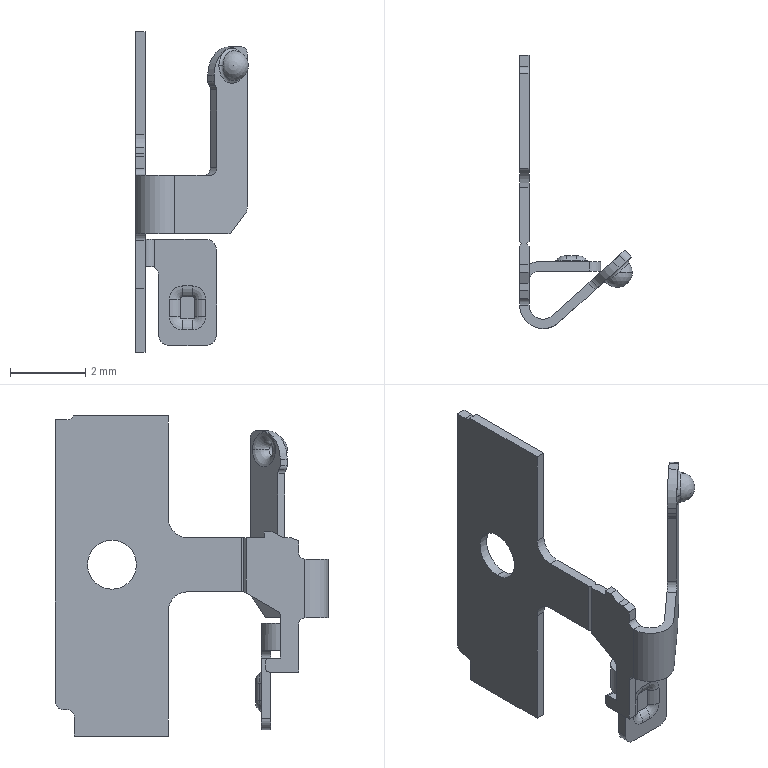Part | NX | 1 solid | 109 faces | box 2.994 x 7.25 x 8.5 mm | volume 11.338 mm3 | plane 50 | cylinder 39 | torus 16 | sphere 4 | commonest cylinder face diameters 0.2 x7 0.4 x7 0.5 x6 0.7 x4 0.6 x3 1 x3